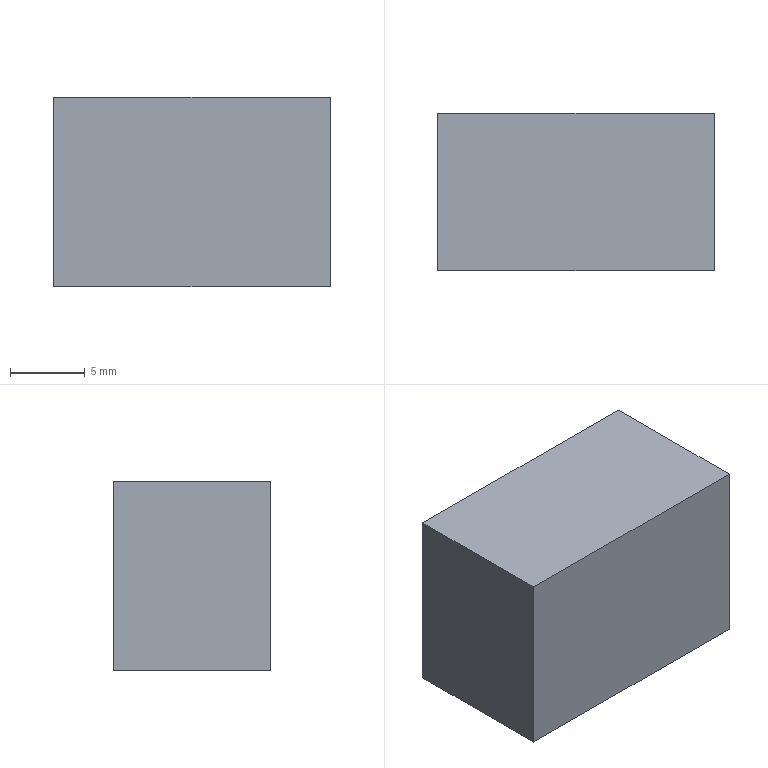Part | STEP file | 0246_Z_102_MXQ12L-30AS-A93_2 | 1 solid | 32 faces | box 18.5 x 10.5 x 12.7 mm | volume 2355 mm3 | plane 24 | cylinder 8 | commonest cylinder face diameters 7 x4 7.5 x4